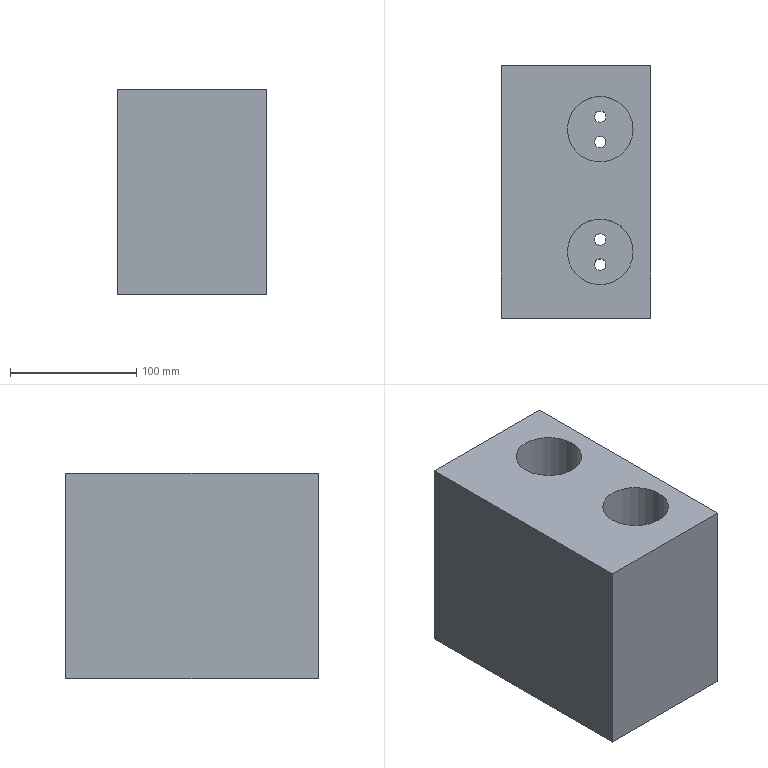Part | NX | features B2-4 2 | 1 solid | 34 faces | box 118 x 200 x 163 mm | volume 3597375 mm3 | cylinder 14 | plane 12 | cone 8 | commonest cylinder face diameters 9 x4 10.5 x4 14.5 x4 52.004 x2
STEP:
#1=CARTESIAN_POINT('',(3080.094,-759.122,570.716));
#2=VERTEX_POINT('',#1);
#3=CARTESIAN_POINT('',(3080.094,-759.122,733.716));
#4=VERTEX_POINT('',#3);
#5=CARTESIAN_POINT('',(3080.094,-759.122,841.216));
#6=DIRECTION('',(0.,0.,1.));
#7=VECTOR('',#6,1000.);
#8=LINE('',#5,#7);
#9=EDGE_CURVE('',#2,#4,#8,.T.);
#10=ORIENTED_EDGE('',*,*,#9,.T.);
#11=CARTESIAN_POINT('',(3080.094,-959.122,733.716));
#12=VERTEX_POINT('',#11);
#13=CARTESIAN_POINT('',(3080.094,-599.122,733.716));
#14=DIRECTION('',(0.,-1.,0.));
#15=VECTOR('',#14,1000.);
#16=LINE('',#13,#15);
#17=EDGE_CURVE('',#4,#12,#16,.T.);
#18=ORIENTED_EDGE('',*,*,#17,.T.);
#19=CARTESIAN_POINT('',(3080.094,-959.122,570.716));
#20=VERTEX_POINT('',#19);
#21=CARTESIAN_POINT('',(3080.094,-959.122,841.216));
#22=DIRECTION('',(0.,0.,-1.));
#23=VECTOR('',#22,1000.);
#24=LINE('',#21,#23);
#25=EDGE_CURVE('',#12,#20,#24,.T.);
#26=ORIENTED_EDGE('',*,*,#25,.T.);
#27=CARTESIAN_POINT('',(3080.094,-599.122,570.716));
#28=DIRECTION('',(0.,-1.,0.));
#29=VECTOR('',#28,1000.);
#30=LINE('',#27,#29);
#31=EDGE_CURVE('',#2,#20,#30,.T.);
#32=ORIENTED_EDGE('',*,*,#31,.F.);
#33=EDGE_LOOP('',(#10,#18,#26,#32));
#34=FACE_BOUND('',#33,.T.);
#35=CARTESIAN_POINT('',(3080.094,-599.122,600.716));
#36=DIRECTION('',(-1.,0.,0.));
#37=DIRECTION('',(0.,0.,1.));
#38=AXIS2_PLACEMENT_3D('',#35,#36,#37);
#39=PLANE('',#38);
#40=ADVANCED_FACE('',(#34),#39,.F.);
#41=CARTESIAN_POINT('',(2972.094,-775.122,570.716));
#42=VERTEX_POINT('',#41);
#43=CARTESIAN_POINT('',(2978.094,-775.122,570.716));
#44=DIRECTION('',(0.,0.,-1.));
#45=DIRECTION('',(-1.,0.,0.));
#46=AXIS2_PLACEMENT_3D('',#43,#44,#45);
#47=CIRCLE('',#46,6.);
#48=EDGE_CURVE('',#42,#42,#47,.T.);
#49=ORIENTED_EDGE('',*,*,#48,.F.);
#50=EDGE_LOOP('',(#49));
#51=FACE_BOUND('',#50,.T.);
#52=CARTESIAN_POINT('',(3058.094,-943.122,570.716));
#53=VERTEX_POINT('',#52);
#54=CARTESIAN_POINT('',(3064.094,-943.122,570.716));
#55=DIRECTION('',(0.,0.,-1.));
#56=DIRECTION('',(-1.,0.,0.));
#57=AXIS2_PLACEMENT_3D('',#54,#55,#56);
#58=CIRCLE('',#57,6.);
#59=EDGE_CURVE('',#53,#53,#58,.T.);
#60=ORIENTED_EDGE('',*,*,#59,.F.);
#61=EDGE_LOOP('',(#60));
#62=FACE_BOUND('',#61,.T.);
#63=CARTESIAN_POINT('',(3058.094,-775.122,570.716));
#64=VERTEX_POINT('',#63);
#65=CARTESIAN_POINT('',(3064.094,-775.122,570.716));
#66=DIRECTION('',(0.,0.,-1.));
#67=DIRECTION('',(-1.,0.,0.));
#68=AXIS2_PLACEMENT_3D('',#65,#66,#67);
#69=CIRCLE('',#68,6.);
#70=EDGE_CURVE('',#64,#64,#69,.T.);
#71=ORIENTED_EDGE('',*,*,#70,.F.);
#72=EDGE_LOOP('',(#71));
#73=FACE_BOUND('',#72,.T.);
#74=CARTESIAN_POINT('',(2972.094,-943.122,570.716));
#75=VERTEX_POINT('',#74);
#76=CARTESIAN_POINT('',(2978.094,-943.122,570.716));
#77=DIRECTION('',(0.,0.,-1.));
#78=DIRECTION('',(-1.,0.,0.));
#79=AXIS2_PLACEMENT_3D('',#76,#77,#78);
#80=CIRCLE('',#79,6.);
#81=EDGE_CURVE('',#75,#75,#80,.T.);
#82=ORIENTED_EDGE('',*,*,#81,.F.);
#83=EDGE_LOOP('',(#82));
#84=FACE_BOUND('',#83,.T.);
#85=CARTESIAN_POINT('',(3033.018,-819.54,570.716));
#86=VERTEX_POINT('',#85);
#87=CARTESIAN_POINT('',(3040.268,-819.54,570.716));
#88=DIRECTION('',(0.,0.,-1.));
#89=DIRECTION('',(-1.,0.,0.));
#90=AXIS2_PLACEMENT_3D('',#87,#88,#89);
#91=CIRCLE('',#90,7.25);
#92=EDGE_CURVE('',#86,#86,#91,.T.);
#93=ORIENTED_EDGE('',*,*,#92,.F.);
#94=EDGE_LOOP('',(#93));
#95=FACE_BOUND('',#94,.T.);
#96=CARTESIAN_POINT('',(3033.018,-799.54,570.716));
#97=VERTEX_POINT('',#96);
#98=CARTESIAN_POINT('',(3040.268,-799.54,570.716));
#99=DIRECTION('',(0.,0.,-1.));
#100=DIRECTION('',(-1.,0.,0.));
#101=AXIS2_PLACEMENT_3D('',#98,#99,#100);
#102=CIRCLE('',#101,7.25);
#103=EDGE_CURVE('',#97,#97,#102,.T.);
#104=ORIENTED_EDGE('',*,*,#103,.F.);
#105=EDGE_LOOP('',(#104));
#106=FACE_BOUND('',#105,.T.);
#107=CARTESIAN_POINT('',(3033.018,-916.709,570.716));
#108=VERTEX_POINT('',#107);
#109=CARTESIAN_POINT('',(3040.268,-916.709,570.716));
#110=DIRECTION('',(0.,0.,-1.));
#111=DIRECTION('',(-1.,0.,0.));
#112=AXIS2_PLACEMENT_3D('',#109,#110,#111);
#113=CIRCLE('',#112,7.25);
#114=EDGE_CURVE('',#108,#108,#113,.T.);
#115=ORIENTED_EDGE('',*,*,#114,.F.);
#116=EDGE_LOOP('',(#115));
#117=FACE_BOUND('',#116,.T.);
#118=CARTESIAN_POINT('',(3033.018,-896.709,570.716));
#119=VERTEX_POINT('',#118);
#120=CARTESIAN_POINT('',(3040.268,-896.709,570.716));
#121=DIRECTION('',(0.,0.,-1.));
#122=DIRECTION('',(-1.,0.,0.));
#123=AXIS2_PLACEMENT_3D('',#120,#121,#122);
#124=CIRCLE('',#123,7.25);
#125=EDGE_CURVE('',#119,#119,#124,.T.);
#126=ORIENTED_EDGE('',*,*,#125,.F.);
#127=EDGE_LOOP('',(#126));
#128=FACE_BOUND('',#127,.T.);
#129=CARTESIAN_POINT('',(2962.094,-759.122,570.716));
#130=VERTEX_POINT('',#129);
#131=CARTESIAN_POINT('',(2962.094,-959.122,570.716));
#132=VERTEX_POINT('',#131);
#133=CARTESIAN_POINT('',(2962.094,0.,570.716));
#134=DIRECTION('',(0.,-1.,0.));
#135=VECTOR('',#134,1000.);
#136=LINE('',#133,#135);
#137=EDGE_CURVE('',#130,#132,#136,.T.);
#138=ORIENTED_EDGE('',*,*,#137,.F.);
#139=CARTESIAN_POINT('',(3160.094,-759.122,570.716));
#140=DIRECTION('',(-1.,0.,0.));
#141=VECTOR('',#140,1000.);
#142=LINE('',#139,#141);
#143=EDGE_CURVE('',#2,#130,#142,.T.);
#144=ORIENTED_EDGE('',*,*,#143,.F.);
#145=ORIENTED_EDGE('',*,*,#31,.T.);
#146=CARTESIAN_POINT('',(3160.094,-959.122,570.716));
#147=DIRECTION('',(1.,0.,0.));
#148=VECTOR('',#147,1000.);
#149=LINE('',#146,#148);
#150=EDGE_CURVE('',#132,#20,#149,.T.);
#151=ORIENTED_EDGE('',*,*,#150,.F.);
#152=EDGE_LOOP('',(#138,#144,#145,#151));
#153=FACE_BOUND('',#152,.T.);
#154=CARTESIAN_POINT('',(-1370.,0.,570.716));
#155=DIRECTION('',(0.,0.,-1.));
#156=DIRECTION('',(-1.,0.,0.));
#157=AXIS2_PLACEMENT_3D('',#154,#155,#156);
#158=PLANE('',#157);
#159=ADVANCED_FACE('',(#51,#62,#73,#84,#95,#106,#117,#128,#153),#158,.T.);
#160=CARTESIAN_POINT('',(3066.268,-809.538,733.716));
#161=VERTEX_POINT('',#160);
#162=CARTESIAN_POINT('',(3040.266,-809.538,733.716));
#163=DIRECTION('',(0.,0.,-1.));
#164=DIRECTION('',(1.,0.,0.));
#165=AXIS2_PLACEMENT_3D('',#162,#163,#164);
#166=CIRCLE('',#165,26.002);
#167=EDGE_CURVE('',#161,#161,#166,.T.);
#168=ORIENTED_EDGE('',*,*,#167,.T.);
#169=EDGE_LOOP('',(#168));
#170=FACE_BOUND('',#169,.T.);
#171=CARTESIAN_POINT('',(3066.268,-906.707,733.716));
#172=VERTEX_POINT('',#171);
#173=CARTESIAN_POINT('',(3040.266,-906.707,733.716));
#174=DIRECTION('',(0.,0.,-1.));
#175=DIRECTION('',(1.,0.,0.));
#176=AXIS2_PLACEMENT_3D('',#173,#174,#175);
#177=CIRCLE('',#176,26.002);
#178=EDGE_CURVE('',#172,#172,#177,.T.);
#179=ORIENTED_EDGE('',*,*,#178,.T.);
#180=EDGE_LOOP('',(#179));
#181=FACE_BOUND('',#180,.T.);
#182=CARTESIAN_POINT('',(2962.094,-759.122,733.716));
#183=VERTEX_POINT('',#182);
#184=CARTESIAN_POINT('',(-1370.,-759.122,733.716));
#185=DIRECTION('',(1.,0.,0.));
#186=VECTOR('',#185,1000.);
#187=LINE('',#184,#186);
#188=EDGE_CURVE('',#183,#4,#187,.T.);
#189=ORIENTED_EDGE('',*,*,#188,.F.);
#190=CARTESIAN_POINT('',(2962.094,-959.122,733.716));
#191=VERTEX_POINT('',#190);
#192=CARTESIAN_POINT('',(2962.094,-859.122,733.716));
#193=DIRECTION('',(0.,1.,0.));
#194=VECTOR('',#193,1000.);
#195=LINE('',#192,#194);
#196=EDGE_CURVE('',#191,#183,#195,.T.);
#197=ORIENTED_EDGE('',*,*,#196,.F.);
#198=CARTESIAN_POINT('',(3160.094,-959.122,733.716));
#199=DIRECTION('',(1.,0.,0.));
#200=VECTOR('',#199,1000.);
#201=LINE('',#198,#200);
#202=EDGE_CURVE('',#191,#12,#201,.T.);
#203=ORIENTED_EDGE('',*,*,#202,.T.);
#204=ORIENTED_EDGE('',*,*,#17,.F.);
#205=EDGE_LOOP('',(#189,#197,#203,#204));
#206=FACE_BOUND('',#205,.T.);
#207=CARTESIAN_POINT('',(-1370.,0.,733.716));
#208=DIRECTION('',(0.,0.,-1.));
#209=DIRECTION('',(-1.,0.,0.));
#210=AXIS2_PLACEMENT_3D('',#207,#208,#209);
#211=PLANE('',#210);
#212=ADVANCED_FACE('',(#170,#181,#206),#211,.F.);
#213=CARTESIAN_POINT('',(2962.094,-759.122,841.216));
#214=DIRECTION('',(0.,0.,-1.));
#215=VECTOR('',#214,1000.);
#216=LINE('',#213,#215);
#217=EDGE_CURVE('',#183,#130,#216,.T.);
#218=ORIENTED_EDGE('',*,*,#217,.T.);
#219=ORIENTED_EDGE('',*,*,#137,.T.);
#220=CARTESIAN_POINT('',(2962.094,-959.122,667.216));
#221=DIRECTION('',(0.,0.,-1.));
#222=VECTOR('',#221,1000.);
#223=LINE('',#220,#222);
#224=EDGE_CURVE('',#191,#132,#223,.T.);
#225=ORIENTED_EDGE('',*,*,#224,.F.);
#226=ORIENTED_EDGE('',*,*,#196,.T.);
#227=EDGE_LOOP('',(#218,#219,#225,#226));
#228=FACE_BOUND('',#227,.T.);
#229=CARTESIAN_POINT('',(2962.094,-859.122,667.216));
#230=DIRECTION('',(1.,0.,0.));
#231=DIRECTION('',(0.,0.,-1.));
#232=AXIS2_PLACEMENT_3D('',#229,#230,#231);
#233=PLANE('',#232);
#234=ADVANCED_FACE('',(#228),#233,.F.);
#235=ORIENTED_EDGE('',*,*,#150,.T.);
#236=ORIENTED_EDGE('',*,*,#25,.F.);
#237=ORIENTED_EDGE('',*,*,#202,.F.);
#238=ORIENTED_EDGE('',*,*,#224,.T.);
#239=EDGE_LOOP('',(#235,#236,#237,#238));
#240=FACE_BOUND('',#239,.T.);
#241=CARTESIAN_POINT('',(3160.094,-959.122,841.216));
#242=DIRECTION('',(0.,-1.,0.));
#243=DIRECTION('',(0.,0.,-1.));
#244=AXIS2_PLACEMENT_3D('',#241,#242,#243);
#245=PLANE('',#244);
#246=ADVANCED_FACE('',(#240),#245,.T.);
#247=ORIENTED_EDGE('',*,*,#188,.T.);
#248=ORIENTED_EDGE('',*,*,#9,.F.);
#249=ORIENTED_EDGE('',*,*,#143,.T.);
#250=ORIENTED_EDGE('',*,*,#217,.F.);
#251=EDGE_LOOP('',(#247,#248,#249,#250));
#252=FACE_BOUND('',#251,.T.);
#253=CARTESIAN_POINT('',(3160.094,-759.122,841.216));
#254=DIRECTION('',(0.,1.,0.));
#255=DIRECTION('',(0.,0.,1.));
#256=AXIS2_PLACEMENT_3D('',#253,#254,#255);
#257=PLANE('',#256);
#258=ADVANCED_FACE('',(#252),#257,.T.);
#259=CARTESIAN_POINT('',(3035.768,-916.709,693.716));
#260=VERTEX_POINT('',#259);
#261=CARTESIAN_POINT('',(3040.268,-916.709,693.716));
#262=DIRECTION('',(0.,0.,-1.));
#263=DIRECTION('',(-1.,0.,0.));
#264=AXIS2_PLACEMENT_3D('',#261,#262,#263);
#265=CIRCLE('',#264,4.5);
#266=EDGE_CURVE('',#260,#260,#265,.T.);
#267=ORIENTED_EDGE('',*,*,#266,.T.);
#268=EDGE_LOOP('',(#267));
#269=FACE_BOUND('',#268,.T.);
#270=CARTESIAN_POINT('',(3035.768,-896.709,693.716));
#271=VERTEX_POINT('',#270);
#272=CARTESIAN_POINT('',(3040.268,-896.709,693.716));
#273=DIRECTION('',(0.,0.,-1.));
#274=DIRECTION('',(-1.,0.,0.));
#275=AXIS2_PLACEMENT_3D('',#272,#273,#274);
#276=CIRCLE('',#275,4.5);
#277=EDGE_CURVE('',#271,#271,#276,.T.);
#278=ORIENTED_EDGE('',*,*,#277,.T.);
#279=EDGE_LOOP('',(#278));
#280=FACE_BOUND('',#279,.T.);
#281=CARTESIAN_POINT('',(3014.264,-906.707,693.716));
#282=VERTEX_POINT('',#281);
#283=CARTESIAN_POINT('',(3040.266,-906.707,693.716));
#284=DIRECTION('',(0.,0.,-1.));
#285=DIRECTION('',(-1.,0.,0.));
#286=AXIS2_PLACEMENT_3D('',#283,#284,#285);
#287=CIRCLE('',#286,26.002);
#288=EDGE_CURVE('',#282,#282,#287,.T.);
#289=ORIENTED_EDGE('',*,*,#288,.F.);
#290=EDGE_LOOP('',(#289));
#291=FACE_BOUND('',#290,.T.);
#292=CARTESIAN_POINT('',(3040.266,-906.707,693.716));
#293=DIRECTION('',(0.,0.,-1.));
#294=DIRECTION('',(-1.,0.,0.));
#295=AXIS2_PLACEMENT_3D('',#292,#293,#294);
#296=PLANE('',#295);
#297=ADVANCED_FACE('',(#269,#280,#291),#296,.F.);
#298=ORIENTED_EDGE('',*,*,#288,.T.);
#299=EDGE_LOOP('',(#298));
#300=FACE_BOUND('',#299,.T.);
#301=ORIENTED_EDGE('',*,*,#178,.F.);
#302=EDGE_LOOP('',(#301));
#303=FACE_BOUND('',#302,.T.);
#304=CARTESIAN_POINT('',(3040.266,-906.707,733.716));
#305=DIRECTION('',(0.,0.,-1.));
#306=DIRECTION('',(1.,0.,0.));
#307=AXIS2_PLACEMENT_3D('',#304,#305,#306);
#308=CYLINDRICAL_SURFACE('',#307,26.002);
#309=ADVANCED_FACE('',(#300,#303),#308,.F.);
#310=CARTESIAN_POINT('',(3035.768,-819.54,693.716));
#311=VERTEX_POINT('',#310);
#312=CARTESIAN_POINT('',(3040.268,-819.54,693.716));
#313=DIRECTION('',(0.,0.,-1.));
#314=DIRECTION('',(-1.,0.,0.));
#315=AXIS2_PLACEMENT_3D('',#312,#313,#314);
#316=CIRCLE('',#315,4.5);
#317=EDGE_CURVE('',#311,#311,#316,.T.);
#318=ORIENTED_EDGE('',*,*,#317,.T.);
#319=EDGE_LOOP('',(#318));
#320=FACE_BOUND('',#319,.T.);
#321=CARTESIAN_POINT('',(3035.768,-799.54,693.716));
#322=VERTEX_POINT('',#321);
#323=CARTESIAN_POINT('',(3040.268,-799.54,693.716));
#324=DIRECTION('',(0.,0.,-1.));
#325=DIRECTION('',(-1.,0.,0.));
#326=AXIS2_PLACEMENT_3D('',#323,#324,#325);
#327=CIRCLE('',#326,4.5);
#328=EDGE_CURVE('',#322,#322,#327,.T.);
#329=ORIENTED_EDGE('',*,*,#328,.T.);
#330=EDGE_LOOP('',(#329));
#331=FACE_BOUND('',#330,.T.);
#332=CARTESIAN_POINT('',(3014.264,-809.538,693.716));
#333=VERTEX_POINT('',#332);
#334=CARTESIAN_POINT('',(3040.266,-809.538,693.716));
#335=DIRECTION('',(0.,0.,-1.));
#336=DIRECTION('',(-1.,0.,0.));
#337=AXIS2_PLACEMENT_3D('',#334,#335,#336);
#338=CIRCLE('',#337,26.002);
#339=EDGE_CURVE('',#333,#333,#338,.T.);
#340=ORIENTED_EDGE('',*,*,#339,.F.);
#341=EDGE_LOOP('',(#340));
#342=FACE_BOUND('',#341,.T.);
#343=CARTESIAN_POINT('',(3040.266,-809.538,693.716));
#344=DIRECTION('',(0.,0.,-1.));
#345=DIRECTION('',(-1.,0.,0.));
#346=AXIS2_PLACEMENT_3D('',#343,#344,#345);
#347=PLANE('',#346);
#348=ADVANCED_FACE('',(#320,#331,#342),#347,.F.);
#349=ORIENTED_EDGE('',*,*,#339,.T.);
#350=EDGE_LOOP('',(#349));
#351=FACE_BOUND('',#350,.T.);
#352=ORIENTED_EDGE('',*,*,#167,.F.);
#353=EDGE_LOOP('',(#352));
#354=FACE_BOUND('',#353,.T.);
#355=CARTESIAN_POINT('',(3040.266,-809.538,733.716));
#356=DIRECTION('',(0.,0.,-1.));
#357=DIRECTION('',(1.,0.,0.));
#358=AXIS2_PLACEMENT_3D('',#355,#356,#357);
#359=CYLINDRICAL_SURFACE('',#358,26.002);
#360=ADVANCED_FACE('',(#351,#354),#359,.F.);
#361=CARTESIAN_POINT('',(3035.768,-896.709,653.716));
#362=VERTEX_POINT('',#361);
#363=CARTESIAN_POINT('',(3040.268,-896.709,653.716));
#364=DIRECTION('',(0.,0.,-1.));
#365=DIRECTION('',(-1.,0.,0.));
#366=AXIS2_PLACEMENT_3D('',#363,#364,#365);
#367=CIRCLE('',#366,4.5);
#368=EDGE_CURVE('',#362,#362,#367,.T.);
#369=ORIENTED_EDGE('',*,*,#368,.T.);
#370=EDGE_LOOP('',(#369));
#371=FACE_BOUND('',#370,.T.);
#372=ORIENTED_EDGE('',*,*,#277,.F.);
#373=EDGE_LOOP('',(#372));
#374=FACE_BOUND('',#373,.T.);
#375=CARTESIAN_POINT('',(3040.268,-896.709,694.716));
#376=DIRECTION('',(0.,0.,-1.));
#377=DIRECTION('',(-1.,0.,0.));
#378=AXIS2_PLACEMENT_3D('',#375,#376,#377);
#379=CYLINDRICAL_SURFACE('',#378,4.5);
#380=ADVANCED_FACE('',(#371,#374),#379,.F.);
#381=ORIENTED_EDGE('',*,*,#125,.T.);
#382=EDGE_LOOP('',(#381));
#383=FACE_BOUND('',#382,.T.);
#384=CARTESIAN_POINT('',(3033.018,-896.709,653.716));
#385=VERTEX_POINT('',#384);
#386=CARTESIAN_POINT('',(3040.268,-896.709,653.716));
#387=DIRECTION('',(0.,0.,-1.));
#388=DIRECTION('',(-1.,0.,0.));
#389=AXIS2_PLACEMENT_3D('',#386,#387,#388);
#390=CIRCLE('',#389,7.25);
#391=EDGE_CURVE('',#385,#385,#390,.F.);
#392=ORIENTED_EDGE('',*,*,#391,.T.);
#393=EDGE_LOOP('',(#392));
#394=FACE_BOUND('',#393,.T.);
#395=CARTESIAN_POINT('',(3040.268,-896.709,653.716));
#396=DIRECTION('',(0.,0.,-1.));
#397=DIRECTION('',(-1.,0.,0.));
#398=AXIS2_PLACEMENT_3D('',#395,#396,#397);
#399=CYLINDRICAL_SURFACE('',#398,7.25);
#400=ADVANCED_FACE('',(#383,#394),#399,.F.);
#401=ORIENTED_EDGE('',*,*,#368,.F.);
#402=EDGE_LOOP('',(#401));
#403=FACE_BOUND('',#402,.T.);
#404=ORIENTED_EDGE('',*,*,#391,.F.);
#405=EDGE_LOOP('',(#404));
#406=FACE_BOUND('',#405,.T.);
#407=CARTESIAN_POINT('',(3040.268,-896.709,653.716));
#408=DIRECTION('',(0.,0.,-1.));
#409=DIRECTION('',(-1.,0.,0.));
#410=AXIS2_PLACEMENT_3D('',#407,#408,#409);
#411=PLANE('',#410);
#412=ADVANCED_FACE('',(#403,#406),#411,.T.);
#413=CARTESIAN_POINT('',(3035.768,-916.709,653.716));
#414=VERTEX_POINT('',#413);
#415=CARTESIAN_POINT('',(3040.268,-916.709,653.716));
#416=DIRECTION('',(0.,0.,-1.));
#417=DIRECTION('',(-1.,0.,0.));
#418=AXIS2_PLACEMENT_3D('',#415,#416,#417);
#419=CIRCLE('',#418,4.5);
#420=EDGE_CURVE('',#414,#414,#419,.T.);
#421=ORIENTED_EDGE('',*,*,#420,.T.);
#422=EDGE_LOOP('',(#421));
#423=FACE_BOUND('',#422,.T.);
#424=ORIENTED_EDGE('',*,*,#266,.F.);
#425=EDGE_LOOP('',(#424));
#426=FACE_BOUND('',#425,.T.);
#427=CARTESIAN_POINT('',(3040.268,-916.709,694.716));
#428=DIRECTION('',(0.,0.,-1.));
#429=DIRECTION('',(-1.,0.,0.));
#430=AXIS2_PLACEMENT_3D('',#427,#428,#429);
#431=CYLINDRICAL_SURFACE('',#430,4.5);
#432=ADVANCED_FACE('',(#423,#426),#431,.F.);
#433=ORIENTED_EDGE('',*,*,#114,.T.);
#434=EDGE_LOOP('',(#433));
#435=FACE_BOUND('',#434,.T.);
#436=CARTESIAN_POINT('',(3033.018,-916.709,653.716));
#437=VERTEX_POINT('',#436);
#438=CARTESIAN_POINT('',(3040.268,-916.709,653.716));
#439=DIRECTION('',(0.,0.,-1.));
#440=DIRECTION('',(-1.,0.,0.));
#441=AXIS2_PLACEMENT_3D('',#438,#439,#440);
#442=CIRCLE('',#441,7.25);
#443=EDGE_CURVE('',#437,#437,#442,.F.);
#444=ORIENTED_EDGE('',*,*,#443,.T.);
#445=EDGE_LOOP('',(#444));
#446=FACE_BOUND('',#445,.T.);
#447=CARTESIAN_POINT('',(3040.268,-916.709,653.716));
#448=DIRECTION('',(0.,0.,-1.));
#449=DIRECTION('',(-1.,0.,0.));
#450=AXIS2_PLACEMENT_3D('',#447,#448,#449);
#451=CYLINDRICAL_SURFACE('',#450,7.25);
#452=ADVANCED_FACE('',(#435,#446),#451,.F.);
#453=ORIENTED_EDGE('',*,*,#420,.F.);
#454=EDGE_LOOP('',(#453));
#455=FACE_BOUND('',#454,.T.);
#456=ORIENTED_EDGE('',*,*,#443,.F.);
#457=EDGE_LOOP('',(#456));
#458=FACE_BOUND('',#457,.T.);
#459=CARTESIAN_POINT('',(3040.268,-916.709,653.716));
#460=DIRECTION('',(0.,0.,-1.));
#461=DIRECTION('',(-1.,0.,0.));
#462=AXIS2_PLACEMENT_3D('',#459,#460,#461);
#463=PLANE('',#462);
#464=ADVANCED_FACE('',(#455,#458),#463,.T.);
#465=CARTESIAN_POINT('',(3035.768,-799.54,653.716));
#466=VERTEX_POINT('',#465);
#467=CARTESIAN_POINT('',(3040.268,-799.54,653.716));
#468=DIRECTION('',(0.,0.,-1.));
#469=DIRECTION('',(-1.,0.,0.));
#470=AXIS2_PLACEMENT_3D('',#467,#468,#469);
#471=CIRCLE('',#470,4.5);
#472=EDGE_CURVE('',#466,#466,#471,.T.);
#473=ORIENTED_EDGE('',*,*,#472,.T.);
#474=EDGE_LOOP('',(#473));
#475=FACE_BOUND('',#474,.T.);
#476=ORIENTED_EDGE('',*,*,#328,.F.);
#477=EDGE_LOOP('',(#476));
#478=FACE_BOUND('',#477,.T.);
#479=CARTESIAN_POINT('',(3040.268,-799.54,694.716));
#480=DIRECTION('',(0.,0.,-1.));
#481=DIRECTION('',(-1.,0.,0.));
#482=AXIS2_PLACEMENT_3D('',#479,#480,#481);
#483=CYLINDRICAL_SURFACE('',#482,4.5);
#484=ADVANCED_FACE('',(#475,#478),#483,.F.);
#485=ORIENTED_EDGE('',*,*,#103,.T.);
#486=EDGE_LOOP('',(#485));
#487=FACE_BOUND('',#486,.T.);
#488=CARTESIAN_POINT('',(3033.018,-799.54,653.716));
#489=VERTEX_POINT('',#488);
#490=CARTESIAN_POINT('',(3040.268,-799.54,653.716));
#491=DIRECTION('',(0.,0.,-1.));
#492=DIRECTION('',(-1.,0.,0.));
#493=AXIS2_PLACEMENT_3D('',#490,#491,#492);
#494=CIRCLE('',#493,7.25);
#495=EDGE_CURVE('',#489,#489,#494,.F.);
#496=ORIENTED_EDGE('',*,*,#495,.T.);
#497=EDGE_LOOP('',(#496));
#498=FACE_BOUND('',#497,.T.);
#499=CARTESIAN_POINT('',(3040.268,-799.54,653.716));
#500=DIRECTION('',(0.,0.,-1.));
#501=DIRECTION('',(-1.,0.,0.));
#502=AXIS2_PLACEMENT_3D('',#499,#500,#501);
#503=CYLINDRICAL_SURFACE('',#502,7.25);
#504=ADVANCED_FACE('',(#487,#498),#503,.F.);
#505=ORIENTED_EDGE('',*,*,#472,.F.);
#506=EDGE_LOOP('',(#505));
#507=FACE_BOUND('',#506,.T.);
#508=ORIENTED_EDGE('',*,*,#495,.F.);
#509=EDGE_LOOP('',(#508));
#510=FACE_BOUND('',#509,.T.);
#511=CARTESIAN_POINT('',(3040.268,-799.54,653.716));
#512=DIRECTION('',(0.,0.,-1.));
#513=DIRECTION('',(-1.,0.,0.));
#514=AXIS2_PLACEMENT_3D('',#511,#512,#513);
#515=PLANE('',#514);
#516=ADVANCED_FACE('',(#507,#510),#515,.T.);
#517=CARTESIAN_POINT('',(3035.768,-819.54,653.716));
#518=VERTEX_POINT('',#517);
#519=CARTESIAN_POINT('',(3040.268,-819.54,653.716));
#520=DIRECTION('',(0.,0.,-1.));
#521=DIRECTION('',(-1.,0.,0.));
#522=AXIS2_PLACEMENT_3D('',#519,#520,#521);
#523=CIRCLE('',#522,4.5);
#524=EDGE_CURVE('',#518,#518,#523,.T.);
#525=ORIENTED_EDGE('',*,*,#524,.T.);
#526=EDGE_LOOP('',(#525));
#527=FACE_BOUND('',#526,.T.);
#528=ORIENTED_EDGE('',*,*,#317,.F.);
#529=EDGE_LOOP('',(#528));
#530=FACE_BOUND('',#529,.T.);
#531=CARTESIAN_POINT('',(3040.268,-819.54,694.716));
#532=DIRECTION('',(0.,0.,-1.));
#533=DIRECTION('',(-1.,0.,0.));
#534=AXIS2_PLACEMENT_3D('',#531,#532,#533);
#535=CYLINDRICAL_SURFACE('',#534,4.5);
#536=ADVANCED_FACE('',(#527,#530),#535,.F.);
#537=ORIENTED_EDGE('',*,*,#92,.T.);
#538=EDGE_LOOP('',(#537));
#539=FACE_BOUND('',#538,.T.);
#540=CARTESIAN_POINT('',(3033.018,-819.54,653.716));
#541=VERTEX_POINT('',#540);
#542=CARTESIAN_POINT('',(3040.268,-819.54,653.716));
#543=DIRECTION('',(0.,0.,-1.));
#544=DIRECTION('',(-1.,0.,0.));
#545=AXIS2_PLACEMENT_3D('',#542,#543,#544);
#546=CIRCLE('',#545,7.25);
#547=EDGE_CURVE('',#541,#541,#546,.F.);
#548=ORIENTED_EDGE('',*,*,#547,.T.);
#549=EDGE_LOOP('',(#548));
#550=FACE_BOUND('',#549,.T.);
#551=CARTESIAN_POINT('',(3040.268,-819.54,653.716));
#552=DIRECTION('',(0.,0.,-1.));
#553=DIRECTION('',(-1.,0.,0.));
#554=AXIS2_PLACEMENT_3D('',#551,#552,#553);
#555=CYLINDRICAL_SURFACE('',#554,7.25);
#556=ADVANCED_FACE('',(#539,#550),#555,.F.);
#557=ORIENTED_EDGE('',*,*,#524,.F.);
#558=EDGE_LOOP('',(#557));
#559=FACE_BOUND('',#558,.T.);
#560=ORIENTED_EDGE('',*,*,#547,.F.);
#561=EDGE_LOOP('',(#560));
#562=FACE_BOUND('',#561,.T.);
#563=CARTESIAN_POINT('',(3040.268,-819.54,653.716));
#564=DIRECTION('',(0.,0.,-1.));
#565=DIRECTION('',(-1.,0.,0.));
#566=AXIS2_PLACEMENT_3D('',#563,#564,#565);
#567=PLANE('',#566);
#568=ADVANCED_FACE('',(#559,#562),#567,.T.);
#569=CARTESIAN_POINT('',(2972.844,-943.122,571.466));
#570=VERTEX_POINT('',#569);
#571=CARTESIAN_POINT('',(2978.094,-943.122,571.466));
#572=DIRECTION('',(0.,0.,-1.));
#573=DIRECTION('',(-1.,0.,0.));
#574=AXIS2_PLACEMENT_3D('',#571,#572,#573);
#575=CIRCLE('',#574,5.25);
#576=EDGE_CURVE('',#570,#570,#575,.F.);
#577=ORIENTED_EDGE('',*,*,#576,.F.);
#578=EDGE_LOOP('',(#577));
#579=FACE_BOUND('',#578,.T.);
#580=CARTESIAN_POINT('',(2972.844,-943.122,610.716));
#581=VERTEX_POINT('',#580);
#582=CARTESIAN_POINT('',(2978.094,-943.122,610.716));
#583=DIRECTION('',(0.,0.,-1.));
#584=DIRECTION('',(-1.,0.,0.));
#585=AXIS2_PLACEMENT_3D('',#582,#583,#584);
#586=CIRCLE('',#585,5.25);
#587=EDGE_CURVE('',#581,#581,#586,.F.);
#588=ORIENTED_EDGE('',*,*,#587,.T.);
#589=EDGE_LOOP('',(#588));
#590=FACE_BOUND('',#589,.T.);
#591=CARTESIAN_POINT('',(2978.094,-943.122,615.966));
#592=DIRECTION('',(0.,0.,-1.));
#593=DIRECTION('',(-1.,0.,0.));
#594=AXIS2_PLACEMENT_3D('',#591,#592,#593);
#595=CYLINDRICAL_SURFACE('',#594,5.25);
#596=ADVANCED_FACE('',(#579,#590),#595,.F.);
#597=CARTESIAN_POINT('',(2978.094,-943.122,615.966));
#598=VERTEX_POINT('',#597);
#599=VERTEX_LOOP('',#598);
#600=FACE_BOUND('',#599,.T.);
#601=ORIENTED_EDGE('',*,*,#587,.F.);
#602=EDGE_LOOP('',(#601));
#603=FACE_BOUND('',#602,.T.);
#604=CARTESIAN_POINT('',(2978.094,-943.122,610.716));
#605=DIRECTION('',(0.,0.,-1.));
#606=DIRECTION('',(-1.,0.,0.));
#607=AXIS2_PLACEMENT_3D('',#604,#605,#606);
#608=CONICAL_SURFACE('',#607,5.25,0.7854);
#609=ADVANCED_FACE('',(#600,#603),#608,.F.);
#610=ORIENTED_EDGE('',*,*,#576,.T.);
#611=EDGE_LOOP('',(#610));
#612=FACE_BOUND('',#611,.T.);
#613=ORIENTED_EDGE('',*,*,#81,.T.);
#614=EDGE_LOOP('',(#613));
#615=FACE_BOUND('',#614,.T.);
#616=CARTESIAN_POINT('',(2978.094,-943.122,570.716));
#617=DIRECTION('',(0.,0.,-1.));
#618=DIRECTION('',(-1.,0.,0.));
#619=AXIS2_PLACEMENT_3D('',#616,#617,#618);
#620=CONICAL_SURFACE('',#619,6.,0.7854);
#621=ADVANCED_FACE('',(#612,#615),#620,.F.);
#622=CARTESIAN_POINT('',(3058.844,-775.122,571.466));
#623=VERTEX_POINT('',#622);
#624=CARTESIAN_POINT('',(3064.094,-775.122,571.466));
#625=DIRECTION('',(0.,0.,-1.));
#626=DIRECTION('',(-1.,0.,0.));
#627=AXIS2_PLACEMENT_3D('',#624,#625,#626);
#628=CIRCLE('',#627,5.25);
#629=EDGE_CURVE('',#623,#623,#628,.F.);
#630=ORIENTED_EDGE('',*,*,#629,.F.);
#631=EDGE_LOOP('',(#630));
#632=FACE_BOUND('',#631,.T.);
#633=CARTESIAN_POINT('',(3058.844,-775.122,610.716));
#634=VERTEX_POINT('',#633);
#635=CARTESIAN_POINT('',(3064.094,-775.122,610.716));
#636=DIRECTION('',(0.,0.,-1.));
#637=DIRECTION('',(-1.,0.,0.));
#638=AXIS2_PLACEMENT_3D('',#635,#636,#637);
#639=CIRCLE('',#638,5.25);
#640=EDGE_CURVE('',#634,#634,#639,.F.);
#641=ORIENTED_EDGE('',*,*,#640,.T.);
#642=EDGE_LOOP('',(#641));
#643=FACE_BOUND('',#642,.T.);
#644=CARTESIAN_POINT('',(3064.094,-775.122,615.966));
#645=DIRECTION('',(0.,0.,-1.));
#646=DIRECTION('',(-1.,0.,0.));
#647=AXIS2_PLACEMENT_3D('',#644,#645,#646);
#648=CYLINDRICAL_SURFACE('',#647,5.25);
#649=ADVANCED_FACE('',(#632,#643),#648,.F.);
#650=CARTESIAN_POINT('',(3064.094,-775.122,615.966));
#651=VERTEX_POINT('',#650);
#652=VERTEX_LOOP('',#651);
#653=FACE_BOUND('',#652,.T.);
#654=ORIENTED_EDGE('',*,*,#640,.F.);
#655=EDGE_LOOP('',(#654));
#656=FACE_BOUND('',#655,.T.);
#657=CARTESIAN_POINT('',(3064.094,-775.122,610.716));
#658=DIRECTION('',(0.,0.,-1.));
#659=DIRECTION('',(-1.,0.,0.));
#660=AXIS2_PLACEMENT_3D('',#657,#658,#659);
#661=CONICAL_SURFACE('',#660,5.25,0.7854);
#662=ADVANCED_FACE('',(#653,#656),#661,.F.);
#663=ORIENTED_EDGE('',*,*,#629,.T.);
#664=EDGE_LOOP('',(#663));
#665=FACE_BOUND('',#664,.T.);
#666=ORIENTED_EDGE('',*,*,#70,.T.);
#667=EDGE_LOOP('',(#666));
#668=FACE_BOUND('',#667,.T.);
#669=CARTESIAN_POINT('',(3064.094,-775.122,570.716));
#670=DIRECTION('',(0.,0.,-1.));
#671=DIRECTION('',(-1.,0.,0.));
#672=AXIS2_PLACEMENT_3D('',#669,#670,#671);
#673=CONICAL_SURFACE('',#672,6.,0.7854);
#674=ADVANCED_FACE('',(#665,#668),#673,.F.);
#675=CARTESIAN_POINT('',(3058.844,-943.122,571.466));
#676=VERTEX_POINT('',#675);
#677=CARTESIAN_POINT('',(3064.094,-943.122,571.466));
#678=DIRECTION('',(0.,0.,-1.));
#679=DIRECTION('',(-1.,0.,0.));
#680=AXIS2_PLACEMENT_3D('',#677,#678,#679);
#681=CIRCLE('',#680,5.25);
#682=EDGE_CURVE('',#676,#676,#681,.F.);
#683=ORIENTED_EDGE('',*,*,#682,.F.);
#684=EDGE_LOOP('',(#683));
#685=FACE_BOUND('',#684,.T.);
#686=CARTESIAN_POINT('',(3058.844,-943.122,610.716));
#687=VERTEX_POINT('',#686);
#688=CARTESIAN_POINT('',(3064.094,-943.122,610.716));
#689=DIRECTION('',(0.,0.,-1.));
#690=DIRECTION('',(-1.,0.,0.));
#691=AXIS2_PLACEMENT_3D('',#688,#689,#690);
#692=CIRCLE('',#691,5.25);
#693=EDGE_CURVE('',#687,#687,#692,.F.);
#694=ORIENTED_EDGE('',*,*,#693,.T.);
#695=EDGE_LOOP('',(#694));
#696=FACE_BOUND('',#695,.T.);
#697=CARTESIAN_POINT('',(3064.094,-943.122,615.966));
#698=DIRECTION('',(0.,0.,-1.));
#699=DIRECTION('',(-1.,0.,0.));
#700=AXIS2_PLACEMENT_3D('',#697,#698,#699);
#701=CYLINDRICAL_SURFACE('',#700,5.25);
#702=ADVANCED_FACE('',(#685,#696),#701,.F.);
#703=CARTESIAN_POINT('',(3064.094,-943.122,615.966));
#704=VERTEX_POINT('',#703);
#705=VERTEX_LOOP('',#704);
#706=FACE_BOUND('',#705,.T.);
#707=ORIENTED_EDGE('',*,*,#693,.F.);
#708=EDGE_LOOP('',(#707));
#709=FACE_BOUND('',#708,.T.);
#710=CARTESIAN_POINT('',(3064.094,-943.122,610.716));
#711=DIRECTION('',(0.,0.,-1.));
#712=DIRECTION('',(-1.,0.,0.));
#713=AXIS2_PLACEMENT_3D('',#710,#711,#712);
#714=CONICAL_SURFACE('',#713,5.25,0.7854);
#715=ADVANCED_FACE('',(#706,#709),#714,.F.);
#716=ORIENTED_EDGE('',*,*,#682,.T.);
#717=EDGE_LOOP('',(#716));
#718=FACE_BOUND('',#717,.T.);
#719=ORIENTED_EDGE('',*,*,#59,.T.);
#720=EDGE_LOOP('',(#719));
#721=FACE_BOUND('',#720,.T.);
#722=CARTESIAN_POINT('',(3064.094,-943.122,570.716));
#723=DIRECTION('',(0.,0.,-1.));
#724=DIRECTION('',(-1.,0.,0.));
#725=AXIS2_PLACEMENT_3D('',#722,#723,#724);
#726=CONICAL_SURFACE('',#725,6.,0.7854);
#727=ADVANCED_FACE('',(#718,#721),#726,.F.);
#728=CARTESIAN_POINT('',(2972.844,-775.122,571.466));
#729=VERTEX_POINT('',#728);
#730=CARTESIAN_POINT('',(2978.094,-775.122,571.466));
#731=DIRECTION('',(0.,0.,-1.));
#732=DIRECTION('',(-1.,0.,0.));
#733=AXIS2_PLACEMENT_3D('',#730,#731,#732);
#734=CIRCLE('',#733,5.25);
#735=EDGE_CURVE('',#729,#729,#734,.F.);
#736=ORIENTED_EDGE('',*,*,#735,.F.);
#737=EDGE_LOOP('',(#736));
#738=FACE_BOUND('',#737,.T.);
#739=CARTESIAN_POINT('',(2972.844,-775.122,610.716));
#740=VERTEX_POINT('',#739);
#741=CARTESIAN_POINT('',(2978.094,-775.122,610.716));
#742=DIRECTION('',(0.,0.,-1.));
#743=DIRECTION('',(-1.,0.,0.));
#744=AXIS2_PLACEMENT_3D('',#741,#742,#743);
#745=CIRCLE('',#744,5.25);
#746=EDGE_CURVE('',#740,#740,#745,.F.);
#747=ORIENTED_EDGE('',*,*,#746,.T.);
#748=EDGE_LOOP('',(#747));
#749=FACE_BOUND('',#748,.T.);
#750=CARTESIAN_POINT('',(2978.094,-775.122,615.966));
#751=DIRECTION('',(0.,0.,-1.));
#752=DIRECTION('',(-1.,0.,0.));
#753=AXIS2_PLACEMENT_3D('',#750,#751,#752);
#754=CYLINDRICAL_SURFACE('',#753,5.25);
#755=ADVANCED_FACE('',(#738,#749),#754,.F.);
#756=CARTESIAN_POINT('',(2978.094,-775.122,615.966));
#757=VERTEX_POINT('',#756);
#758=VERTEX_LOOP('',#757);
#759=FACE_BOUND('',#758,.T.);
#760=ORIENTED_EDGE('',*,*,#746,.F.);
#761=EDGE_LOOP('',(#760));
#762=FACE_BOUND('',#761,.T.);
#763=CARTESIAN_POINT('',(2978.094,-775.122,610.716));
#764=DIRECTION('',(0.,0.,-1.));
#765=DIRECTION('',(-1.,0.,0.));
#766=AXIS2_PLACEMENT_3D('',#763,#764,#765);
#767=CONICAL_SURFACE('',#766,5.25,0.7854);
#768=ADVANCED_FACE('',(#759,#762),#767,.F.);
#769=ORIENTED_EDGE('',*,*,#735,.T.);
#770=EDGE_LOOP('',(#769));
#771=FACE_BOUND('',#770,.T.);
#772=ORIENTED_EDGE('',*,*,#48,.T.);
#773=EDGE_LOOP('',(#772));
#774=FACE_BOUND('',#773,.T.);
#775=CARTESIAN_POINT('',(2978.094,-775.122,570.716));
#776=DIRECTION('',(0.,0.,-1.));
#777=DIRECTION('',(-1.,0.,0.));
#778=AXIS2_PLACEMENT_3D('',#775,#776,#777);
#779=CONICAL_SURFACE('',#778,6.,0.7854);
#780=ADVANCED_FACE('',(#771,#774),#779,.F.);
#781=CLOSED_SHELL('',(#40,#159,#212,#234,#246,#258,#297,#309,#348,#360,#380,#400,#412,#432,#452,#464,#484,#504,#516,#536,#556,#568,#596,#609,#621,#649,#662,#674,#702,#715,#727,#755,#768,#780));
#782=MANIFOLD_SOLID_BREP('',#781);
#783=(LENGTH_UNIT()NAMED_UNIT(*)SI_UNIT(.MILLI.,.METRE.));
#784=UNCERTAINTY_MEASURE_WITH_UNIT(LENGTH_MEASURE(0.00001),#783,'','');
#785=(NAMED_UNIT(*)PLANE_ANGLE_UNIT()SI_UNIT($,.RADIAN.));
#786=(NAMED_UNIT(*)SI_UNIT($,.STERADIAN.)SOLID_ANGLE_UNIT());
#787=(GEOMETRIC_REPRESENTATION_CONTEXT(3)GLOBAL_UNCERTAINTY_ASSIGNED_CONTEXT((#784))GLOBAL_UNIT_ASSIGNED_CONTEXT((#783,#785,#786))REPRESENTATION_CONTEXT('',''));
#788=ADVANCED_BREP_SHAPE_REPRESENTATION('',(#782),#787);